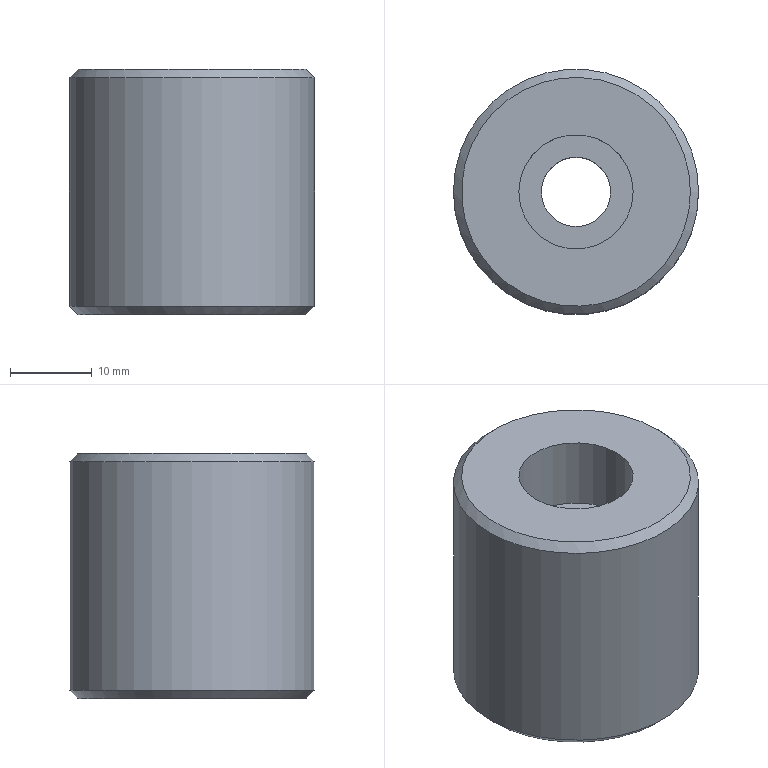Part | STEP file | solid 78 | 1 solid | 8 faces | box 30 x 30 x 30 mm | volume 18536 mm3 | plane 3 | cylinder 3 | cone 2 | commonest cylinder face diameters 8.5 x1 14 x1 30 x1